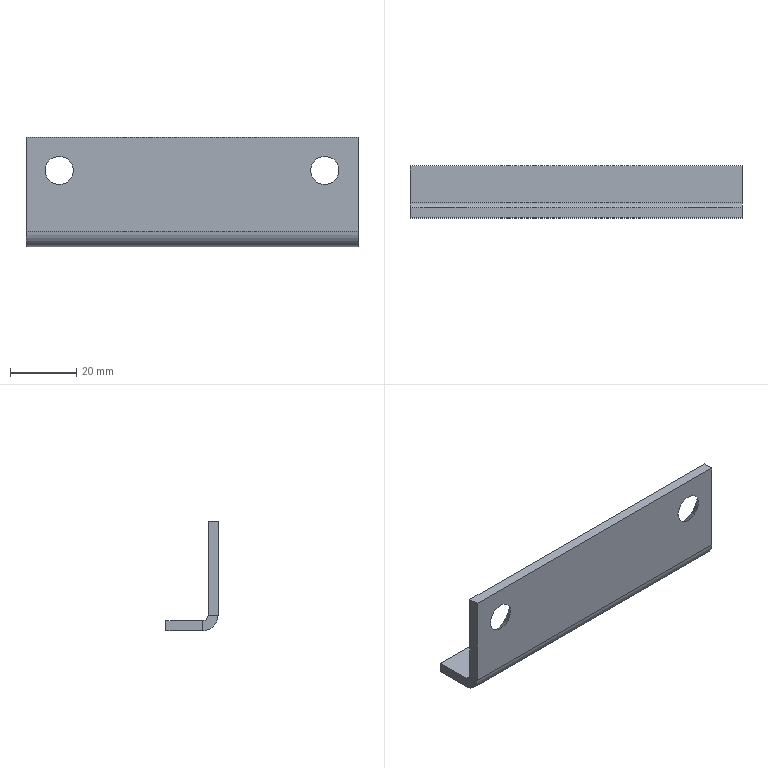Part | NX | features BREP 1 | 1 solid | 18 faces | box 100.076 x 15.723 x 32.995 mm | volume 12820 mm3 | plane 12 | cone 4 | cylinder 2 | commonest cylinder face diameters 3.175 x1 9.22 x1
STEP:
#1=CARTESIAN_POINT('',(50.038,0.,0.));
#2=VERTEX_POINT('',#1);
#3=CARTESIAN_POINT('',(50.038,0.,-28.384));
#4=VERTEX_POINT('',#3);
#5=CARTESIAN_POINT('',(50.038,0.,0.));
#6=DIRECTION('',(0.,0.,-1.));
#7=VECTOR('',#6,1000.);
#8=LINE('',#5,#7);
#9=EDGE_CURVE('',#2,#4,#8,.T.);
#10=ORIENTED_EDGE('',*,*,#9,.T.);
#11=CARTESIAN_POINT('',(-50.038,0.,-28.384));
#12=VERTEX_POINT('',#11);
#13=CARTESIAN_POINT('',(50.038,0.,-28.384));
#14=DIRECTION('',(-1.,0.,0.));
#15=VECTOR('',#14,1000.);
#16=LINE('',#13,#15);
#17=EDGE_CURVE('',#4,#12,#16,.T.);
#18=ORIENTED_EDGE('',*,*,#17,.T.);
#19=CARTESIAN_POINT('',(-50.038,0.,0.));
#20=VERTEX_POINT('',#19);
#21=CARTESIAN_POINT('',(-50.038,0.,-28.384));
#22=DIRECTION('',(0.,0.,1.));
#23=VECTOR('',#22,1000.);
#24=LINE('',#21,#23);
#25=EDGE_CURVE('',#12,#20,#24,.T.);
#26=ORIENTED_EDGE('',*,*,#25,.T.);
#27=CARTESIAN_POINT('',(-50.038,0.,0.));
#28=DIRECTION('',(1.,0.,0.));
#29=VECTOR('',#28,1000.);
#30=LINE('',#27,#29);
#31=EDGE_CURVE('',#20,#2,#30,.T.);
#32=ORIENTED_EDGE('',*,*,#31,.T.);
#33=EDGE_LOOP('',(#10,#18,#26,#32));
#34=FACE_BOUND('',#33,.T.);
#35=CARTESIAN_POINT('',(33.148,0.,-10.008));
#36=VERTEX_POINT('',#35);
#37=CARTESIAN_POINT('',(46.912,0.,-10.008));
#38=VERTEX_POINT('',#37);
#39=CARTESIAN_POINT('',(40.03,0.,-10.008));
#40=DIRECTION('',(0.,1.,0.));
#41=DIRECTION('',(-1.,0.,0.));
#42=AXIS2_PLACEMENT_3D('',#39,#40,#41);
#43=CIRCLE('',#42,6.882);
#44=EDGE_CURVE('',#36,#38,#43,.T.);
#45=ORIENTED_EDGE('',*,*,#44,.F.);
#46=CARTESIAN_POINT('',(40.03,0.,-10.008));
#47=DIRECTION('',(0.,1.,0.));
#48=DIRECTION('',(1.,0.,0.));
#49=AXIS2_PLACEMENT_3D('',#46,#47,#48);
#50=CIRCLE('',#49,6.882);
#51=EDGE_CURVE('',#38,#36,#50,.T.);
#52=ORIENTED_EDGE('',*,*,#51,.F.);
#53=EDGE_LOOP('',(#45,#52));
#54=FACE_BOUND('',#53,.T.);
#55=CARTESIAN_POINT('',(-46.912,0.,-10.008));
#56=VERTEX_POINT('',#55);
#57=CARTESIAN_POINT('',(-33.148,0.,-10.008));
#58=VERTEX_POINT('',#57);
#59=CARTESIAN_POINT('',(-40.03,0.,-10.008));
#60=DIRECTION('',(0.,1.,0.));
#61=DIRECTION('',(-1.,0.,0.));
#62=AXIS2_PLACEMENT_3D('',#59,#60,#61);
#63=CIRCLE('',#62,6.882);
#64=EDGE_CURVE('',#56,#58,#63,.T.);
#65=ORIENTED_EDGE('',*,*,#64,.F.);
#66=CARTESIAN_POINT('',(-40.03,0.,-10.008));
#67=DIRECTION('',(0.,1.,0.));
#68=DIRECTION('',(1.,0.,0.));
#69=AXIS2_PLACEMENT_3D('',#66,#67,#68);
#70=CIRCLE('',#69,6.882);
#71=EDGE_CURVE('',#58,#56,#70,.T.);
#72=ORIENTED_EDGE('',*,*,#71,.F.);
#73=EDGE_LOOP('',(#65,#72));
#74=FACE_BOUND('',#73,.T.);
#75=CARTESIAN_POINT('',(0.,0.,0.));
#76=DIRECTION('',(0.,1.,0.));
#77=DIRECTION('',(1.,0.,0.));
#78=AXIS2_PLACEMENT_3D('',#75,#76,#77);
#79=PLANE('',#78);
#80=ADVANCED_FACE('',(#34,#54,#74),#79,.T.);
#81=CARTESIAN_POINT('',(-50.038,-3.023,0.));
#82=VERTEX_POINT('',#81);
#83=CARTESIAN_POINT('',(-50.038,0.,0.));
#84=DIRECTION('',(0.,-1.,0.));
#85=VECTOR('',#84,1000.);
#86=LINE('',#83,#85);
#87=EDGE_CURVE('',#20,#82,#86,.T.);
#88=ORIENTED_EDGE('',*,*,#87,.T.);
#89=CARTESIAN_POINT('',(50.038,-3.023,0.));
#90=VERTEX_POINT('',#89);
#91=CARTESIAN_POINT('',(-50.038,-3.023,0.));
#92=DIRECTION('',(1.,0.,0.));
#93=VECTOR('',#92,1000.);
#94=LINE('',#91,#93);
#95=EDGE_CURVE('',#82,#90,#94,.T.);
#96=ORIENTED_EDGE('',*,*,#95,.T.);
#97=CARTESIAN_POINT('',(50.038,0.,0.));
#98=DIRECTION('',(0.,-1.,0.));
#99=VECTOR('',#98,1000.);
#100=LINE('',#97,#99);
#101=EDGE_CURVE('',#2,#90,#100,.T.);
#102=ORIENTED_EDGE('',*,*,#101,.F.);
#103=ORIENTED_EDGE('',*,*,#31,.F.);
#104=EDGE_LOOP('',(#88,#96,#102,#103));
#105=FACE_BOUND('',#104,.T.);
#106=CARTESIAN_POINT('',(0.,-1.511,0.));
#107=DIRECTION('',(0.,0.,1.));
#108=DIRECTION('',(1.,0.,0.));
#109=AXIS2_PLACEMENT_3D('',#106,#107,#108);
#110=PLANE('',#109);
#111=ADVANCED_FACE('',(#105),#110,.T.);
#112=ORIENTED_EDGE('',*,*,#101,.T.);
#113=CARTESIAN_POINT('',(50.038,-3.023,-28.384));
#114=VERTEX_POINT('',#113);
#115=CARTESIAN_POINT('',(50.038,-3.023,0.));
#116=DIRECTION('',(0.,0.,-1.));
#117=VECTOR('',#116,1000.);
#118=LINE('',#115,#117);
#119=EDGE_CURVE('',#90,#114,#118,.T.);
#120=ORIENTED_EDGE('',*,*,#119,.T.);
#121=CARTESIAN_POINT('',(50.038,0.,-28.384));
#122=DIRECTION('',(0.,-1.,0.));
#123=VECTOR('',#122,1000.);
#124=LINE('',#121,#123);
#125=EDGE_CURVE('',#4,#114,#124,.T.);
#126=ORIENTED_EDGE('',*,*,#125,.F.);
#127=ORIENTED_EDGE('',*,*,#9,.F.);
#128=EDGE_LOOP('',(#112,#120,#126,#127));
#129=FACE_BOUND('',#128,.T.);
#130=CARTESIAN_POINT('',(50.038,-1.511,-14.986));
#131=DIRECTION('',(1.,0.,0.));
#132=DIRECTION('',(0.,1.,0.));
#133=AXIS2_PLACEMENT_3D('',#130,#131,#132);
#134=PLANE('',#133);
#135=ADVANCED_FACE('',(#129),#134,.T.);
#136=ORIENTED_EDGE('',*,*,#125,.T.);
#137=CARTESIAN_POINT('',(50.038,1.587,-32.995));
#138=VERTEX_POINT('',#137);
#139=CARTESIAN_POINT('',(50.038,1.587,-28.384));
#140=DIRECTION('',(-1.,0.,0.));
#141=DIRECTION('',(0.,0.,-1.));
#142=AXIS2_PLACEMENT_3D('',#139,#140,#141);
#143=CIRCLE('',#142,4.61);
#144=EDGE_CURVE('',#138,#114,#143,.T.);
#145=ORIENTED_EDGE('',*,*,#144,.F.);
#146=CARTESIAN_POINT('',(50.038,1.587,-29.972));
#147=VERTEX_POINT('',#146);
#148=CARTESIAN_POINT('',(50.038,1.587,-29.972));
#149=DIRECTION('',(0.,0.,-1.));
#150=VECTOR('',#149,1000.);
#151=LINE('',#148,#150);
#152=EDGE_CURVE('',#147,#138,#151,.T.);
#153=ORIENTED_EDGE('',*,*,#152,.F.);
#154=CARTESIAN_POINT('',(50.038,1.587,-28.384));
#155=DIRECTION('',(-1.,0.,0.));
#156=DIRECTION('',(0.,0.,-1.));
#157=AXIS2_PLACEMENT_3D('',#154,#155,#156);
#158=CIRCLE('',#157,1.587);
#159=EDGE_CURVE('',#147,#4,#158,.T.);
#160=ORIENTED_EDGE('',*,*,#159,.T.);
#161=EDGE_LOOP('',(#136,#145,#153,#160));
#162=FACE_BOUND('',#161,.T.);
#163=CARTESIAN_POINT('',(50.038,-0.6037,-30.576));
#164=DIRECTION('',(-1.,0.,0.));
#165=DIRECTION('',(0.,0.,1.));
#166=AXIS2_PLACEMENT_3D('',#163,#164,#165);
#167=PLANE('',#166);
#168=ADVANCED_FACE('',(#162),#167,.F.);
#169=CARTESIAN_POINT('',(-50.038,1.587,-29.972));
#170=VERTEX_POINT('',#169);
#171=CARTESIAN_POINT('',(-50.038,1.587,-28.384));
#172=DIRECTION('',(-1.,0.,0.));
#173=DIRECTION('',(0.,0.,-1.));
#174=AXIS2_PLACEMENT_3D('',#171,#172,#173);
#175=CIRCLE('',#174,1.587);
#176=EDGE_CURVE('',#170,#12,#175,.T.);
#177=ORIENTED_EDGE('',*,*,#176,.T.);
#178=ORIENTED_EDGE('',*,*,#17,.F.);
#179=ORIENTED_EDGE('',*,*,#159,.F.);
#180=CARTESIAN_POINT('',(50.038,1.587,-29.972));
#181=DIRECTION('',(-1.,0.,0.));
#182=VECTOR('',#181,1000.);
#183=LINE('',#180,#182);
#184=EDGE_CURVE('',#147,#170,#183,.T.);
#185=ORIENTED_EDGE('',*,*,#184,.T.);
#186=EDGE_LOOP('',(#177,#178,#179,#185));
#187=FACE_BOUND('',#186,.T.);
#188=CARTESIAN_POINT('',(50.038,1.587,-28.384));
#189=DIRECTION('',(-1.,0.,0.));
#190=DIRECTION('',(0.,0.,-1.));
#191=AXIS2_PLACEMENT_3D('',#188,#189,#190);
#192=CYLINDRICAL_SURFACE('',#191,1.587);
#193=ADVANCED_FACE('',(#187),#192,.F.);
#194=ORIENTED_EDGE('',*,*,#184,.F.);
#195=CARTESIAN_POINT('',(50.038,12.7,-29.972));
#196=VERTEX_POINT('',#195);
#197=CARTESIAN_POINT('',(50.038,12.7,-29.972));
#198=DIRECTION('',(0.,-1.,0.));
#199=VECTOR('',#198,1000.);
#200=LINE('',#197,#199);
#201=EDGE_CURVE('',#196,#147,#200,.T.);
#202=ORIENTED_EDGE('',*,*,#201,.F.);
#203=CARTESIAN_POINT('',(-50.038,12.7,-29.972));
#204=VERTEX_POINT('',#203);
#205=CARTESIAN_POINT('',(-50.038,12.7,-29.972));
#206=DIRECTION('',(1.,0.,0.));
#207=VECTOR('',#206,1000.);
#208=LINE('',#205,#207);
#209=EDGE_CURVE('',#204,#196,#208,.T.);
#210=ORIENTED_EDGE('',*,*,#209,.F.);
#211=CARTESIAN_POINT('',(-50.038,1.587,-29.972));
#212=DIRECTION('',(0.,1.,0.));
#213=VECTOR('',#212,1000.);
#214=LINE('',#211,#213);
#215=EDGE_CURVE('',#170,#204,#214,.T.);
#216=ORIENTED_EDGE('',*,*,#215,.F.);
#217=EDGE_LOOP('',(#194,#202,#210,#216));
#218=FACE_BOUND('',#217,.T.);
#219=CARTESIAN_POINT('',(26.26,0.,-29.972));
#220=DIRECTION('',(0.,0.,-1.));
#221=DIRECTION('',(0.,-1.,0.));
#222=AXIS2_PLACEMENT_3D('',#219,#220,#221);
#223=PLANE('',#222);
#224=ADVANCED_FACE('',(#218),#223,.F.);
#225=CARTESIAN_POINT('',(-50.038,12.7,-32.995));
#226=VERTEX_POINT('',#225);
#227=CARTESIAN_POINT('',(-50.038,12.7,-29.972));
#228=DIRECTION('',(0.,0.,-1.));
#229=VECTOR('',#228,1000.);
#230=LINE('',#227,#229);
#231=EDGE_CURVE('',#204,#226,#230,.T.);
#232=ORIENTED_EDGE('',*,*,#231,.T.);
#233=CARTESIAN_POINT('',(-50.038,1.587,-32.995));
#234=VERTEX_POINT('',#233);
#235=CARTESIAN_POINT('',(-50.038,1.587,-32.995));
#236=DIRECTION('',(0.,1.,0.));
#237=VECTOR('',#236,1000.);
#238=LINE('',#235,#237);
#239=EDGE_CURVE('',#234,#226,#238,.T.);
#240=ORIENTED_EDGE('',*,*,#239,.F.);
#241=CARTESIAN_POINT('',(-50.038,1.587,-29.972));
#242=DIRECTION('',(0.,0.,-1.));
#243=VECTOR('',#242,1000.);
#244=LINE('',#241,#243);
#245=EDGE_CURVE('',#170,#234,#244,.T.);
#246=ORIENTED_EDGE('',*,*,#245,.F.);
#247=ORIENTED_EDGE('',*,*,#215,.T.);
#248=EDGE_LOOP('',(#232,#240,#246,#247));
#249=FACE_BOUND('',#248,.T.);
#250=CARTESIAN_POINT('',(-50.038,7.144,-31.483));
#251=DIRECTION('',(1.,0.,0.));
#252=DIRECTION('',(0.,1.,0.));
#253=AXIS2_PLACEMENT_3D('',#250,#251,#252);
#254=PLANE('',#253);
#255=ADVANCED_FACE('',(#249),#254,.F.);
#256=ORIENTED_EDGE('',*,*,#245,.T.);
#257=CARTESIAN_POINT('',(-50.038,-3.023,-28.384));
#258=VERTEX_POINT('',#257);
#259=CARTESIAN_POINT('',(-50.038,1.587,-28.384));
#260=DIRECTION('',(-1.,0.,0.));
#261=DIRECTION('',(0.,0.,-1.));
#262=AXIS2_PLACEMENT_3D('',#259,#260,#261);
#263=CIRCLE('',#262,4.61);
#264=EDGE_CURVE('',#234,#258,#263,.T.);
#265=ORIENTED_EDGE('',*,*,#264,.T.);
#266=CARTESIAN_POINT('',(-50.038,0.,-28.384));
#267=DIRECTION('',(0.,-1.,0.));
#268=VECTOR('',#267,1000.);
#269=LINE('',#266,#268);
#270=EDGE_CURVE('',#12,#258,#269,.T.);
#271=ORIENTED_EDGE('',*,*,#270,.F.);
#272=ORIENTED_EDGE('',*,*,#176,.F.);
#273=EDGE_LOOP('',(#256,#265,#271,#272));
#274=FACE_BOUND('',#273,.T.);
#275=CARTESIAN_POINT('',(-50.038,-0.6037,-30.576));
#276=DIRECTION('',(-1.,0.,0.));
#277=DIRECTION('',(0.,0.,1.));
#278=AXIS2_PLACEMENT_3D('',#275,#276,#277);
#279=PLANE('',#278);
#280=ADVANCED_FACE('',(#274),#279,.T.);
#281=ORIENTED_EDGE('',*,*,#270,.T.);
#282=CARTESIAN_POINT('',(-50.038,-3.023,-28.384));
#283=DIRECTION('',(0.,0.,1.));
#284=VECTOR('',#283,1000.);
#285=LINE('',#282,#284);
#286=EDGE_CURVE('',#258,#82,#285,.T.);
#287=ORIENTED_EDGE('',*,*,#286,.T.);
#288=ORIENTED_EDGE('',*,*,#87,.F.);
#289=ORIENTED_EDGE('',*,*,#25,.F.);
#290=EDGE_LOOP('',(#281,#287,#288,#289));
#291=FACE_BOUND('',#290,.T.);
#292=CARTESIAN_POINT('',(-50.038,-1.511,-14.986));
#293=DIRECTION('',(-1.,0.,0.));
#294=DIRECTION('',(0.,0.,1.));
#295=AXIS2_PLACEMENT_3D('',#292,#293,#294);
#296=PLANE('',#295);
#297=ADVANCED_FACE('',(#291),#296,.T.);
#298=ORIENTED_EDGE('',*,*,#286,.F.);
#299=CARTESIAN_POINT('',(50.038,-3.023,-28.384));
#300=DIRECTION('',(-1.,0.,0.));
#301=VECTOR('',#300,1000.);
#302=LINE('',#299,#301);
#303=EDGE_CURVE('',#114,#258,#302,.T.);
#304=ORIENTED_EDGE('',*,*,#303,.F.);
#305=ORIENTED_EDGE('',*,*,#119,.F.);
#306=ORIENTED_EDGE('',*,*,#95,.F.);
#307=EDGE_LOOP('',(#298,#304,#305,#306));
#308=FACE_BOUND('',#307,.T.);
#309=CARTESIAN_POINT('',(35.776,-3.023,-10.008));
#310=VERTEX_POINT('',#309);
#311=CARTESIAN_POINT('',(44.285,-3.023,-10.008));
#312=VERTEX_POINT('',#311);
#313=CARTESIAN_POINT('',(40.03,-3.023,-10.008));
#314=DIRECTION('',(0.,1.,0.));
#315=DIRECTION('',(-1.,0.,0.));
#316=AXIS2_PLACEMENT_3D('',#313,#314,#315);
#317=CIRCLE('',#316,4.255);
#318=EDGE_CURVE('',#310,#312,#317,.T.);
#319=ORIENTED_EDGE('',*,*,#318,.T.);
#320=CARTESIAN_POINT('',(40.03,-3.023,-10.008));
#321=DIRECTION('',(0.,1.,0.));
#322=DIRECTION('',(1.,0.,0.));
#323=AXIS2_PLACEMENT_3D('',#320,#321,#322);
#324=CIRCLE('',#323,4.255);
#325=EDGE_CURVE('',#312,#310,#324,.T.);
#326=ORIENTED_EDGE('',*,*,#325,.T.);
#327=EDGE_LOOP('',(#319,#326));
#328=FACE_BOUND('',#327,.T.);
#329=CARTESIAN_POINT('',(-44.285,-3.023,-10.008));
#330=VERTEX_POINT('',#329);
#331=CARTESIAN_POINT('',(-35.776,-3.023,-10.008));
#332=VERTEX_POINT('',#331);
#333=CARTESIAN_POINT('',(-40.03,-3.023,-10.008));
#334=DIRECTION('',(0.,1.,0.));
#335=DIRECTION('',(-1.,0.,0.));
#336=AXIS2_PLACEMENT_3D('',#333,#334,#335);
#337=CIRCLE('',#336,4.255);
#338=EDGE_CURVE('',#330,#332,#337,.T.);
#339=ORIENTED_EDGE('',*,*,#338,.T.);
#340=CARTESIAN_POINT('',(-40.03,-3.023,-10.008));
#341=DIRECTION('',(0.,1.,0.));
#342=DIRECTION('',(1.,0.,0.));
#343=AXIS2_PLACEMENT_3D('',#340,#341,#342);
#344=CIRCLE('',#343,4.255);
#345=EDGE_CURVE('',#332,#330,#344,.T.);
#346=ORIENTED_EDGE('',*,*,#345,.T.);
#347=EDGE_LOOP('',(#339,#346));
#348=FACE_BOUND('',#347,.T.);
#349=CARTESIAN_POINT('',(0.,-3.023,0.));
#350=DIRECTION('',(0.,1.,0.));
#351=DIRECTION('',(1.,0.,0.));
#352=AXIS2_PLACEMENT_3D('',#349,#350,#351);
#353=PLANE('',#352);
#354=ADVANCED_FACE('',(#308,#328,#348),#353,.F.);
#355=ORIENTED_EDGE('',*,*,#144,.T.);
#356=ORIENTED_EDGE('',*,*,#303,.T.);
#357=ORIENTED_EDGE('',*,*,#264,.F.);
#358=CARTESIAN_POINT('',(50.038,1.587,-32.995));
#359=DIRECTION('',(-1.,0.,0.));
#360=VECTOR('',#359,1000.);
#361=LINE('',#358,#360);
#362=EDGE_CURVE('',#138,#234,#361,.T.);
#363=ORIENTED_EDGE('',*,*,#362,.F.);
#364=EDGE_LOOP('',(#355,#356,#357,#363));
#365=FACE_BOUND('',#364,.T.);
#366=CARTESIAN_POINT('',(50.038,1.587,-28.384));
#367=DIRECTION('',(-1.,0.,0.));
#368=DIRECTION('',(0.,0.,-1.));
#369=AXIS2_PLACEMENT_3D('',#366,#367,#368);
#370=CYLINDRICAL_SURFACE('',#369,4.61);
#371=ADVANCED_FACE('',(#365),#370,.T.);
#372=CARTESIAN_POINT('',(50.038,12.7,-32.995));
#373=VERTEX_POINT('',#372);
#374=CARTESIAN_POINT('',(-50.038,12.7,-32.995));
#375=DIRECTION('',(1.,0.,0.));
#376=VECTOR('',#375,1000.);
#377=LINE('',#374,#376);
#378=EDGE_CURVE('',#226,#373,#377,.T.);
#379=ORIENTED_EDGE('',*,*,#378,.T.);
#380=CARTESIAN_POINT('',(50.038,12.7,-32.995));
#381=DIRECTION('',(0.,-1.,0.));
#382=VECTOR('',#381,1000.);
#383=LINE('',#380,#382);
#384=EDGE_CURVE('',#373,#138,#383,.T.);
#385=ORIENTED_EDGE('',*,*,#384,.T.);
#386=ORIENTED_EDGE('',*,*,#362,.T.);
#387=ORIENTED_EDGE('',*,*,#239,.T.);
#388=EDGE_LOOP('',(#379,#385,#386,#387));
#389=FACE_BOUND('',#388,.T.);
#390=CARTESIAN_POINT('',(26.26,0.,-32.995));
#391=DIRECTION('',(0.,0.,-1.));
#392=DIRECTION('',(0.,-1.,0.));
#393=AXIS2_PLACEMENT_3D('',#390,#391,#392);
#394=PLANE('',#393);
#395=ADVANCED_FACE('',(#389),#394,.T.);
#396=ORIENTED_EDGE('',*,*,#152,.T.);
#397=ORIENTED_EDGE('',*,*,#384,.F.);
#398=CARTESIAN_POINT('',(50.038,12.7,-29.972));
#399=DIRECTION('',(0.,0.,-1.));
#400=VECTOR('',#399,1000.);
#401=LINE('',#398,#400);
#402=EDGE_CURVE('',#196,#373,#401,.T.);
#403=ORIENTED_EDGE('',*,*,#402,.F.);
#404=ORIENTED_EDGE('',*,*,#201,.T.);
#405=EDGE_LOOP('',(#396,#397,#403,#404));
#406=FACE_BOUND('',#405,.T.);
#407=CARTESIAN_POINT('',(50.038,7.144,-31.483));
#408=DIRECTION('',(-1.,0.,0.));
#409=DIRECTION('',(0.,0.,1.));
#410=AXIS2_PLACEMENT_3D('',#407,#408,#409);
#411=PLANE('',#410);
#412=ADVANCED_FACE('',(#406),#411,.F.);
#413=ORIENTED_EDGE('',*,*,#402,.T.);
#414=ORIENTED_EDGE('',*,*,#378,.F.);
#415=ORIENTED_EDGE('',*,*,#231,.F.);
#416=ORIENTED_EDGE('',*,*,#209,.T.);
#417=EDGE_LOOP('',(#413,#414,#415,#416));
#418=FACE_BOUND('',#417,.T.);
#419=CARTESIAN_POINT('',(0.,12.7,-31.483));
#420=DIRECTION('',(0.,-1.,0.));
#421=DIRECTION('',(0.,0.,-1.));
#422=AXIS2_PLACEMENT_3D('',#419,#420,#421);
#423=PLANE('',#422);
#424=ADVANCED_FACE('',(#418),#423,.F.);
#425=CARTESIAN_POINT('',(35.776,-3.023,-10.008));
#426=DIRECTION('',(-0.6561,0.7547,0.));
#427=VECTOR('',#426,1000.);
#428=LINE('',#425,#427);
#429=EDGE_CURVE('',#310,#36,#428,.T.);
#430=ORIENTED_EDGE('',*,*,#429,.F.);
#431=ORIENTED_EDGE('',*,*,#325,.F.);
#432=CARTESIAN_POINT('',(44.285,-3.023,-10.008));
#433=DIRECTION('',(0.6561,0.7547,0.));
#434=VECTOR('',#433,1000.);
#435=LINE('',#432,#434);
#436=EDGE_CURVE('',#312,#38,#435,.T.);
#437=ORIENTED_EDGE('',*,*,#436,.T.);
#438=ORIENTED_EDGE('',*,*,#51,.T.);
#439=EDGE_LOOP('',(#430,#431,#437,#438));
#440=FACE_BOUND('',#439,.T.);
#441=CARTESIAN_POINT('',(40.03,-1.511,-10.008));
#442=DIRECTION('',(0.,1.,0.));
#443=DIRECTION('',(1.,0.,0.));
#444=AXIS2_PLACEMENT_3D('',#441,#442,#443);
#445=CONICAL_SURFACE('',#444,5.568,0.7156);
#446=ADVANCED_FACE('',(#440),#445,.F.);
#447=ORIENTED_EDGE('',*,*,#436,.F.);
#448=ORIENTED_EDGE('',*,*,#318,.F.);
#449=ORIENTED_EDGE('',*,*,#429,.T.);
#450=ORIENTED_EDGE('',*,*,#44,.T.);
#451=EDGE_LOOP('',(#447,#448,#449,#450));
#452=FACE_BOUND('',#451,.T.);
#453=CARTESIAN_POINT('',(40.03,-1.511,-10.008));
#454=DIRECTION('',(0.,1.,0.));
#455=DIRECTION('',(1.,0.,0.));
#456=AXIS2_PLACEMENT_3D('',#453,#454,#455);
#457=CONICAL_SURFACE('',#456,5.568,0.7156);
#458=ADVANCED_FACE('',(#452),#457,.F.);
#459=CARTESIAN_POINT('',(-44.285,-3.023,-10.008));
#460=DIRECTION('',(-0.6561,0.7547,0.));
#461=VECTOR('',#460,1000.);
#462=LINE('',#459,#461);
#463=EDGE_CURVE('',#330,#56,#462,.T.);
#464=ORIENTED_EDGE('',*,*,#463,.F.);
#465=ORIENTED_EDGE('',*,*,#345,.F.);
#466=CARTESIAN_POINT('',(-35.776,-3.023,-10.008));
#467=DIRECTION('',(0.6561,0.7547,0.));
#468=VECTOR('',#467,1000.);
#469=LINE('',#466,#468);
#470=EDGE_CURVE('',#332,#58,#469,.T.);
#471=ORIENTED_EDGE('',*,*,#470,.T.);
#472=ORIENTED_EDGE('',*,*,#71,.T.);
#473=EDGE_LOOP('',(#464,#465,#471,#472));
#474=FACE_BOUND('',#473,.T.);
#475=CARTESIAN_POINT('',(-40.03,-1.511,-10.008));
#476=DIRECTION('',(0.,1.,0.));
#477=DIRECTION('',(1.,0.,0.));
#478=AXIS2_PLACEMENT_3D('',#475,#476,#477);
#479=CONICAL_SURFACE('',#478,5.568,0.7156);
#480=ADVANCED_FACE('',(#474),#479,.F.);
#481=ORIENTED_EDGE('',*,*,#470,.F.);
#482=ORIENTED_EDGE('',*,*,#338,.F.);
#483=ORIENTED_EDGE('',*,*,#463,.T.);
#484=ORIENTED_EDGE('',*,*,#64,.T.);
#485=EDGE_LOOP('',(#481,#482,#483,#484));
#486=FACE_BOUND('',#485,.T.);
#487=CARTESIAN_POINT('',(-40.03,-1.511,-10.008));
#488=DIRECTION('',(0.,1.,0.));
#489=DIRECTION('',(1.,0.,0.));
#490=AXIS2_PLACEMENT_3D('',#487,#488,#489);
#491=CONICAL_SURFACE('',#490,5.568,0.7156);
#492=ADVANCED_FACE('',(#486),#491,.F.);
#493=CLOSED_SHELL('',(#80,#111,#135,#168,#193,#224,#255,#280,#297,#354,#371,#395,#412,#424,#446,#458,#480,#492));
#494=MANIFOLD_SOLID_BREP('',#493);
#495=(LENGTH_UNIT()NAMED_UNIT(*)SI_UNIT(.MILLI.,.METRE.));
#496=UNCERTAINTY_MEASURE_WITH_UNIT(LENGTH_MEASURE(0.00001),#495,'','');
#497=(NAMED_UNIT(*)PLANE_ANGLE_UNIT()SI_UNIT($,.RADIAN.));
#498=(NAMED_UNIT(*)SI_UNIT($,.STERADIAN.)SOLID_ANGLE_UNIT());
#499=(GEOMETRIC_REPRESENTATION_CONTEXT(3)GLOBAL_UNCERTAINTY_ASSIGNED_CONTEXT((#496))GLOBAL_UNIT_ASSIGNED_CONTEXT((#495,#497,#498))REPRESENTATION_CONTEXT('',''));
#500=ADVANCED_BREP_SHAPE_REPRESENTATION('',(#494),#499);